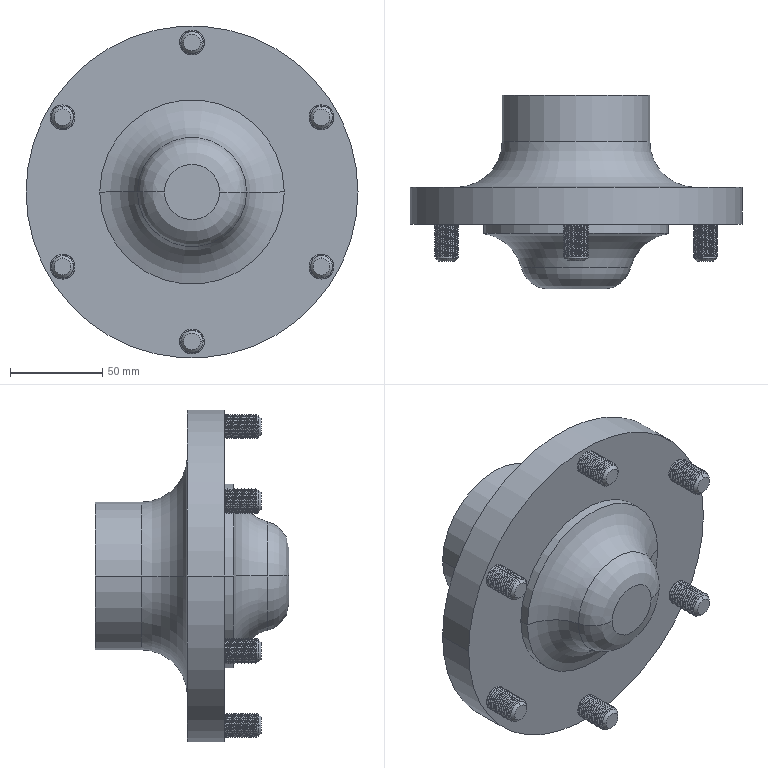Part | SolidWorks | 1 solid | 247 faces | box 180 x 105 x 180 mm | volume 867546 mm3 | cylinder 194 | spline 18 | plane 17 | cone 12 | torus 6 | commonest cylinder face diameters 12 x186 60 x2 80 x2 100 x2 180 x2